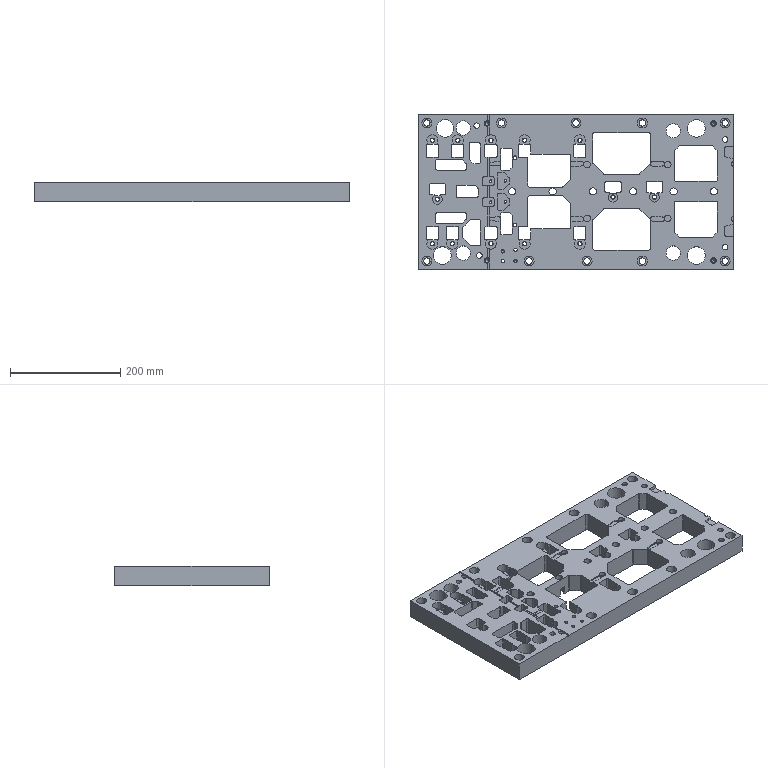Part | NX | features DIE-4 2 | 1 solid | 584 faces | box 570 x 280 x 35.032 mm | volume 3496506 mm3 | cylinder 256 | plane 247 | spline 56 | cone 25 | commonest cylinder face diameters 4 x56 6 x52 5 x20 18 x20 6.806 x17 1 x12